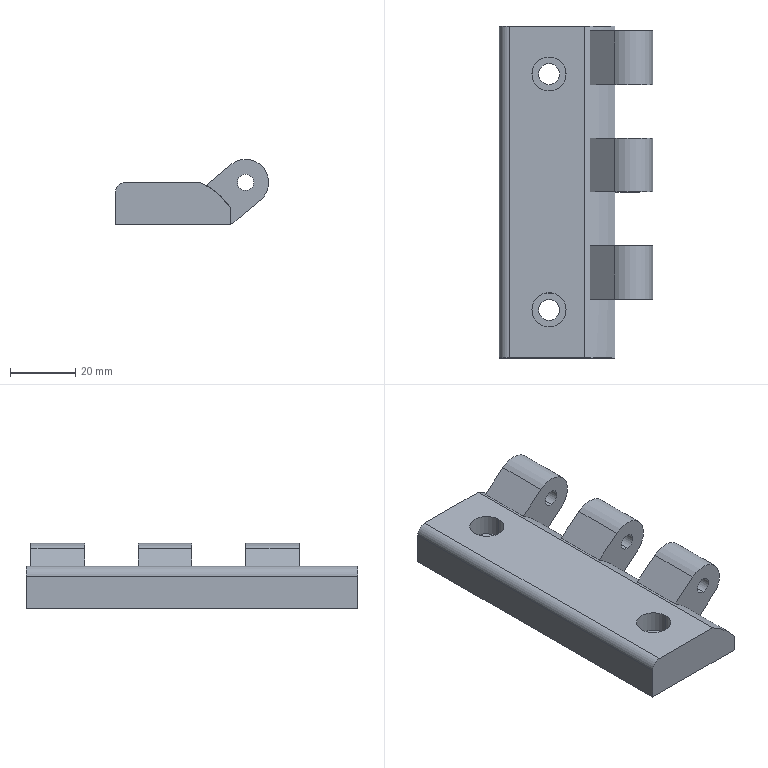Part | SolidWorks | features MBimport 1 | 1 solid | 42 faces | box 47.1 x 102 x 20.1 mm | volume 51608 mm3 | plane 23 | cylinder 19 | commonest cylinder face diameters 5 x6 6.5 x4 10.5 x4 14.2 x3 6 x1 49.62 x1
STEP:
#1=CARTESIAN_POINT('',(-28.,-36.25,-6.5));
#2=VERTEX_POINT('',#1);
#3=CARTESIAN_POINT('',(-21.5,-36.25,-6.5));
#4=VERTEX_POINT('',#3);
#5=CARTESIAN_POINT('',(-24.75,-36.25,-6.5));
#6=DIRECTION('',(0.,0.,-1.));
#7=DIRECTION('',(-1.,0.,0.));
#8=AXIS2_PLACEMENT_3D('',#5,#6,#7);
#9=CIRCLE('',#8,3.25);
#10=EDGE_CURVE('',#2,#4,#9,.T.);
#11=ORIENTED_EDGE('',*,*,#10,.F.);
#12=CARTESIAN_POINT('',(-28.,-36.25,-13.));
#13=VERTEX_POINT('',#12);
#14=CARTESIAN_POINT('',(-28.,-36.25,0.));
#15=DIRECTION('',(0.,0.,-1.));
#16=VECTOR('',#15,1000.);
#17=LINE('',#14,#16);
#18=EDGE_CURVE('',#2,#13,#17,.T.);
#19=ORIENTED_EDGE('',*,*,#18,.T.);
#20=CARTESIAN_POINT('',(-21.5,-36.25,-13.));
#21=VERTEX_POINT('',#20);
#22=CARTESIAN_POINT('',(-24.75,-36.25,-13.));
#23=DIRECTION('',(0.,0.,1.));
#24=DIRECTION('',(1.,0.,0.));
#25=AXIS2_PLACEMENT_3D('',#22,#23,#24);
#26=CIRCLE('',#25,3.25);
#27=EDGE_CURVE('',#21,#13,#26,.T.);
#28=ORIENTED_EDGE('',*,*,#27,.F.);
#29=CARTESIAN_POINT('',(-21.5,-36.25,0.));
#30=DIRECTION('',(0.,0.,-1.));
#31=VECTOR('',#30,1000.);
#32=LINE('',#29,#31);
#33=EDGE_CURVE('',#4,#21,#32,.T.);
#34=ORIENTED_EDGE('',*,*,#33,.F.);
#35=EDGE_LOOP('',(#11,#19,#28,#34));
#36=FACE_OUTER_BOUND('',#35,.T.);
#37=CARTESIAN_POINT('',(-24.75,-36.25,0.));
#38=DIRECTION('',(0.,0.,-1.));
#39=DIRECTION('',(1.,0.,0.));
#40=AXIS2_PLACEMENT_3D('',#37,#38,#39);
#41=CYLINDRICAL_SURFACE('',#40,3.25);
#42=ADVANCED_FACE('',(#36),#41,.F.);
#43=CARTESIAN_POINT('',(-28.,36.25,-6.5));
#44=VERTEX_POINT('',#43);
#45=CARTESIAN_POINT('',(-21.5,36.25,-6.5));
#46=VERTEX_POINT('',#45);
#47=CARTESIAN_POINT('',(-24.75,36.25,-6.5));
#48=DIRECTION('',(0.,0.,-1.));
#49=DIRECTION('',(-1.,0.,0.));
#50=AXIS2_PLACEMENT_3D('',#47,#48,#49);
#51=CIRCLE('',#50,3.25);
#52=EDGE_CURVE('',#44,#46,#51,.T.);
#53=ORIENTED_EDGE('',*,*,#52,.F.);
#54=CARTESIAN_POINT('',(-28.,36.25,-13.));
#55=VERTEX_POINT('',#54);
#56=CARTESIAN_POINT('',(-28.,36.25,0.));
#57=DIRECTION('',(0.,0.,-1.));
#58=VECTOR('',#57,1000.);
#59=LINE('',#56,#58);
#60=EDGE_CURVE('',#44,#55,#59,.T.);
#61=ORIENTED_EDGE('',*,*,#60,.T.);
#62=CARTESIAN_POINT('',(-21.5,36.25,-13.));
#63=VERTEX_POINT('',#62);
#64=CARTESIAN_POINT('',(-24.75,36.25,-13.));
#65=DIRECTION('',(0.,0.,1.));
#66=DIRECTION('',(1.,0.,0.));
#67=AXIS2_PLACEMENT_3D('',#64,#65,#66);
#68=CIRCLE('',#67,3.25);
#69=EDGE_CURVE('',#63,#55,#68,.T.);
#70=ORIENTED_EDGE('',*,*,#69,.F.);
#71=CARTESIAN_POINT('',(-21.5,36.25,0.));
#72=DIRECTION('',(0.,0.,-1.));
#73=VECTOR('',#72,1000.);
#74=LINE('',#71,#73);
#75=EDGE_CURVE('',#46,#63,#74,.T.);
#76=ORIENTED_EDGE('',*,*,#75,.F.);
#77=EDGE_LOOP('',(#53,#61,#70,#76));
#78=FACE_OUTER_BOUND('',#77,.T.);
#79=CARTESIAN_POINT('',(-24.75,36.25,0.));
#80=DIRECTION('',(0.,0.,-1.));
#81=DIRECTION('',(1.,0.,0.));
#82=AXIS2_PLACEMENT_3D('',#79,#80,#81);
#83=CYLINDRICAL_SURFACE('',#82,3.25);
#84=ADVANCED_FACE('',(#78),#83,.F.);
#85=CARTESIAN_POINT('',(-30.,-36.25,0.));
#86=VERTEX_POINT('',#85);
#87=CARTESIAN_POINT('',(-19.5,-36.25,0.));
#88=VERTEX_POINT('',#87);
#89=CARTESIAN_POINT('',(-24.75,-36.25,0.));
#90=DIRECTION('',(0.,0.,-1.));
#91=DIRECTION('',(1.,0.,0.));
#92=AXIS2_PLACEMENT_3D('',#89,#90,#91);
#93=CIRCLE('',#92,5.25);
#94=EDGE_CURVE('',#86,#88,#93,.T.);
#95=ORIENTED_EDGE('',*,*,#94,.F.);
#96=CARTESIAN_POINT('',(-30.,-36.25,-6.5));
#97=VERTEX_POINT('',#96);
#98=CARTESIAN_POINT('',(-30.,-36.25,0.));
#99=DIRECTION('',(0.,0.,-1.));
#100=VECTOR('',#99,1000.);
#101=LINE('',#98,#100);
#102=EDGE_CURVE('',#86,#97,#101,.T.);
#103=ORIENTED_EDGE('',*,*,#102,.T.);
#104=CARTESIAN_POINT('',(-19.5,-36.25,-6.5));
#105=VERTEX_POINT('',#104);
#106=CARTESIAN_POINT('',(-24.75,-36.25,-6.5));
#107=DIRECTION('',(0.,0.,1.));
#108=DIRECTION('',(1.,0.,0.));
#109=AXIS2_PLACEMENT_3D('',#106,#107,#108);
#110=CIRCLE('',#109,5.25);
#111=EDGE_CURVE('',#105,#97,#110,.T.);
#112=ORIENTED_EDGE('',*,*,#111,.F.);
#113=CARTESIAN_POINT('',(-19.5,-36.25,0.));
#114=DIRECTION('',(0.,0.,-1.));
#115=VECTOR('',#114,1000.);
#116=LINE('',#113,#115);
#117=EDGE_CURVE('',#88,#105,#116,.T.);
#118=ORIENTED_EDGE('',*,*,#117,.F.);
#119=EDGE_LOOP('',(#95,#103,#112,#118));
#120=FACE_OUTER_BOUND('',#119,.T.);
#121=CARTESIAN_POINT('',(-24.75,-36.25,0.));
#122=DIRECTION('',(0.,0.,-1.));
#123=DIRECTION('',(1.,0.,0.));
#124=AXIS2_PLACEMENT_3D('',#121,#122,#123);
#125=CYLINDRICAL_SURFACE('',#124,5.25);
#126=ADVANCED_FACE('',(#120),#125,.F.);
#127=CARTESIAN_POINT('',(-30.,36.25,0.));
#128=VERTEX_POINT('',#127);
#129=CARTESIAN_POINT('',(-19.5,36.25,0.));
#130=VERTEX_POINT('',#129);
#131=CARTESIAN_POINT('',(-24.75,36.25,0.));
#132=DIRECTION('',(0.,0.,-1.));
#133=DIRECTION('',(1.,0.,0.));
#134=AXIS2_PLACEMENT_3D('',#131,#132,#133);
#135=CIRCLE('',#134,5.25);
#136=EDGE_CURVE('',#128,#130,#135,.T.);
#137=ORIENTED_EDGE('',*,*,#136,.F.);
#138=CARTESIAN_POINT('',(-30.,36.25,-6.5));
#139=VERTEX_POINT('',#138);
#140=CARTESIAN_POINT('',(-30.,36.25,0.));
#141=DIRECTION('',(0.,0.,-1.));
#142=VECTOR('',#141,1000.);
#143=LINE('',#140,#142);
#144=EDGE_CURVE('',#128,#139,#143,.T.);
#145=ORIENTED_EDGE('',*,*,#144,.T.);
#146=CARTESIAN_POINT('',(-19.5,36.25,-6.5));
#147=VERTEX_POINT('',#146);
#148=CARTESIAN_POINT('',(-24.75,36.25,-6.5));
#149=DIRECTION('',(0.,0.,1.));
#150=DIRECTION('',(1.,0.,0.));
#151=AXIS2_PLACEMENT_3D('',#148,#149,#150);
#152=CIRCLE('',#151,5.25);
#153=EDGE_CURVE('',#147,#139,#152,.T.);
#154=ORIENTED_EDGE('',*,*,#153,.F.);
#155=CARTESIAN_POINT('',(-19.5,36.25,0.));
#156=DIRECTION('',(0.,0.,-1.));
#157=VECTOR('',#156,1000.);
#158=LINE('',#155,#157);
#159=EDGE_CURVE('',#130,#147,#158,.T.);
#160=ORIENTED_EDGE('',*,*,#159,.F.);
#161=EDGE_LOOP('',(#137,#145,#154,#160));
#162=FACE_OUTER_BOUND('',#161,.T.);
#163=CARTESIAN_POINT('',(-24.75,36.25,0.));
#164=DIRECTION('',(0.,0.,-1.));
#165=DIRECTION('',(1.,0.,0.));
#166=AXIS2_PLACEMENT_3D('',#163,#164,#165);
#167=CYLINDRICAL_SURFACE('',#166,5.25);
#168=ADVANCED_FACE('',(#162),#167,.F.);
#169=CARTESIAN_POINT('',(0.,49.5,-2.5));
#170=VERTEX_POINT('',#169);
#171=CARTESIAN_POINT('',(0.,49.5,2.5));
#172=VERTEX_POINT('',#171);
#173=CARTESIAN_POINT('',(0.,49.5,0.));
#174=DIRECTION('',(0.,1.,0.));
#175=DIRECTION('',(1.,0.,0.));
#176=AXIS2_PLACEMENT_3D('',#173,#174,#175);
#177=CIRCLE('',#176,2.5);
#178=EDGE_CURVE('',#170,#172,#177,.T.);
#179=ORIENTED_EDGE('',*,*,#178,.T.);
#180=CARTESIAN_POINT('',(0.,33.,2.5));
#181=VERTEX_POINT('',#180);
#182=CARTESIAN_POINT('',(0.,49.5,2.5));
#183=DIRECTION('',(0.,-1.,0.));
#184=VECTOR('',#183,1000.);
#185=LINE('',#182,#184);
#186=EDGE_CURVE('',#172,#181,#185,.T.);
#187=ORIENTED_EDGE('',*,*,#186,.T.);
#188=CARTESIAN_POINT('',(0.,33.,-2.5));
#189=VERTEX_POINT('',#188);
#190=CARTESIAN_POINT('',(0.,33.,0.));
#191=DIRECTION('',(0.,1.,0.));
#192=DIRECTION('',(1.,0.,0.));
#193=AXIS2_PLACEMENT_3D('',#190,#191,#192);
#194=CIRCLE('',#193,2.5);
#195=EDGE_CURVE('',#189,#181,#194,.T.);
#196=ORIENTED_EDGE('',*,*,#195,.F.);
#197=CARTESIAN_POINT('',(0.,49.5,-2.5));
#198=DIRECTION('',(0.,-1.,0.));
#199=VECTOR('',#198,1000.);
#200=LINE('',#197,#199);
#201=EDGE_CURVE('',#170,#189,#200,.T.);
#202=ORIENTED_EDGE('',*,*,#201,.F.);
#203=EDGE_LOOP('',(#179,#187,#196,#202));
#204=FACE_OUTER_BOUND('',#203,.T.);
#205=CARTESIAN_POINT('',(0.,49.5,0.));
#206=DIRECTION('',(0.,-1.,0.));
#207=DIRECTION('',(0.,0.,-1.));
#208=AXIS2_PLACEMENT_3D('',#205,#206,#207);
#209=CYLINDRICAL_SURFACE('',#208,2.5);
#210=ADVANCED_FACE('',(#204),#209,.F.);
#211=CARTESIAN_POINT('',(0.,16.5,-2.5));
#212=VERTEX_POINT('',#211);
#213=CARTESIAN_POINT('',(0.,16.5,2.5));
#214=VERTEX_POINT('',#213);
#215=CARTESIAN_POINT('',(0.,16.5,0.));
#216=DIRECTION('',(0.,1.,0.));
#217=DIRECTION('',(1.,0.,0.));
#218=AXIS2_PLACEMENT_3D('',#215,#216,#217);
#219=CIRCLE('',#218,2.5);
#220=EDGE_CURVE('',#212,#214,#219,.T.);
#221=ORIENTED_EDGE('',*,*,#220,.T.);
#222=CARTESIAN_POINT('',(0.,0.,2.5));
#223=VERTEX_POINT('',#222);
#224=CARTESIAN_POINT('',(0.,16.5,2.5));
#225=DIRECTION('',(0.,-1.,0.));
#226=VECTOR('',#225,1000.);
#227=LINE('',#224,#226);
#228=EDGE_CURVE('',#214,#223,#227,.T.);
#229=ORIENTED_EDGE('',*,*,#228,.T.);
#230=CARTESIAN_POINT('',(0.,0.,-2.5));
#231=VERTEX_POINT('',#230);
#232=CARTESIAN_POINT('',(0.,0.,0.));
#233=DIRECTION('',(0.,1.,0.));
#234=DIRECTION('',(1.,0.,0.));
#235=AXIS2_PLACEMENT_3D('',#232,#233,#234);
#236=CIRCLE('',#235,2.5);
#237=EDGE_CURVE('',#231,#223,#236,.T.);
#238=ORIENTED_EDGE('',*,*,#237,.F.);
#239=CARTESIAN_POINT('',(0.,16.5,-2.5));
#240=DIRECTION('',(0.,-1.,0.));
#241=VECTOR('',#240,1000.);
#242=LINE('',#239,#241);
#243=EDGE_CURVE('',#212,#231,#242,.T.);
#244=ORIENTED_EDGE('',*,*,#243,.F.);
#245=EDGE_LOOP('',(#221,#229,#238,#244));
#246=FACE_OUTER_BOUND('',#245,.T.);
#247=CARTESIAN_POINT('',(0.,16.5,0.));
#248=DIRECTION('',(0.,-1.,0.));
#249=DIRECTION('',(0.,0.,-1.));
#250=AXIS2_PLACEMENT_3D('',#247,#248,#249);
#251=CYLINDRICAL_SURFACE('',#250,2.5);
#252=ADVANCED_FACE('',(#246),#251,.F.);
#253=CARTESIAN_POINT('',(0.,-16.5,-2.5));
#254=VERTEX_POINT('',#253);
#255=CARTESIAN_POINT('',(0.,-16.5,2.5));
#256=VERTEX_POINT('',#255);
#257=CARTESIAN_POINT('',(0.,-16.5,0.));
#258=DIRECTION('',(0.,1.,0.));
#259=DIRECTION('',(1.,0.,0.));
#260=AXIS2_PLACEMENT_3D('',#257,#258,#259);
#261=CIRCLE('',#260,2.5);
#262=EDGE_CURVE('',#254,#256,#261,.T.);
#263=ORIENTED_EDGE('',*,*,#262,.T.);
#264=CARTESIAN_POINT('',(0.,-33.,2.5));
#265=VERTEX_POINT('',#264);
#266=CARTESIAN_POINT('',(0.,-16.5,2.5));
#267=DIRECTION('',(0.,-1.,0.));
#268=VECTOR('',#267,1000.);
#269=LINE('',#266,#268);
#270=EDGE_CURVE('',#256,#265,#269,.T.);
#271=ORIENTED_EDGE('',*,*,#270,.T.);
#272=CARTESIAN_POINT('',(0.,-33.,-2.5));
#273=VERTEX_POINT('',#272);
#274=CARTESIAN_POINT('',(0.,-33.,0.));
#275=DIRECTION('',(0.,1.,0.));
#276=DIRECTION('',(1.,0.,0.));
#277=AXIS2_PLACEMENT_3D('',#274,#275,#276);
#278=CIRCLE('',#277,2.5);
#279=EDGE_CURVE('',#273,#265,#278,.T.);
#280=ORIENTED_EDGE('',*,*,#279,.F.);
#281=CARTESIAN_POINT('',(0.,-16.5,-2.5));
#282=DIRECTION('',(0.,-1.,0.));
#283=VECTOR('',#282,1000.);
#284=LINE('',#281,#283);
#285=EDGE_CURVE('',#254,#273,#284,.T.);
#286=ORIENTED_EDGE('',*,*,#285,.F.);
#287=EDGE_LOOP('',(#263,#271,#280,#286));
#288=FACE_OUTER_BOUND('',#287,.T.);
#289=CARTESIAN_POINT('',(0.,-16.5,0.));
#290=DIRECTION('',(0.,-1.,0.));
#291=DIRECTION('',(0.,0.,-1.));
#292=AXIS2_PLACEMENT_3D('',#289,#290,#291);
#293=CYLINDRICAL_SURFACE('',#292,2.5);
#294=ADVANCED_FACE('',(#288),#293,.F.);
#295=CARTESIAN_POINT('',(-4.5,49.5,-7.958));
#296=VERTEX_POINT('',#295);
#297=CARTESIAN_POINT('',(-12.154,49.5,-0.8929));
#298=VERTEX_POINT('',#297);
#299=CARTESIAN_POINT('',(-24.78,49.5,-22.25));
#300=DIRECTION('',(0.,-1.,0.));
#301=DIRECTION('',(1.,0.,0.));
#302=AXIS2_PLACEMENT_3D('',#299,#300,#301);
#303=CIRCLE('',#302,24.81);
#304=EDGE_CURVE('',#296,#298,#303,.T.);
#305=ORIENTED_EDGE('',*,*,#304,.F.);
#306=CARTESIAN_POINT('',(-4.5,51.,-7.958));
#307=VERTEX_POINT('',#306);
#308=CARTESIAN_POINT('',(-4.5,-51.,-7.958));
#309=DIRECTION('',(0.,1.,0.));
#310=VECTOR('',#309,1000.);
#311=LINE('',#308,#310);
#312=EDGE_CURVE('',#296,#307,#311,.T.);
#313=ORIENTED_EDGE('',*,*,#312,.T.);
#314=CARTESIAN_POINT('',(-13.804,51.,0.));
#315=VERTEX_POINT('',#314);
#316=CARTESIAN_POINT('',(-24.78,51.,-22.25));
#317=DIRECTION('',(0.,-1.,0.));
#318=DIRECTION('',(1.,0.,0.));
#319=AXIS2_PLACEMENT_3D('',#316,#317,#318);
#320=CIRCLE('',#319,24.81);
#321=EDGE_CURVE('',#307,#315,#320,.T.);
#322=ORIENTED_EDGE('',*,*,#321,.T.);
#323=CARTESIAN_POINT('',(-13.804,-51.,0.));
#324=VERTEX_POINT('',#323);
#325=CARTESIAN_POINT('',(-13.804,-51.,0.));
#326=DIRECTION('',(0.,1.,0.));
#327=VECTOR('',#326,1000.);
#328=LINE('',#325,#327);
#329=EDGE_CURVE('',#324,#315,#328,.T.);
#330=ORIENTED_EDGE('',*,*,#329,.F.);
#331=CARTESIAN_POINT('',(-4.5,-51.,-7.958));
#332=VERTEX_POINT('',#331);
#333=CARTESIAN_POINT('',(-24.78,-51.,-22.25));
#334=DIRECTION('',(0.,-1.,0.));
#335=DIRECTION('',(1.,0.,0.));
#336=AXIS2_PLACEMENT_3D('',#333,#334,#335);
#337=CIRCLE('',#336,24.81);
#338=EDGE_CURVE('',#332,#324,#337,.T.);
#339=ORIENTED_EDGE('',*,*,#338,.F.);
#340=CARTESIAN_POINT('',(-4.5,-33.,-7.958));
#341=VERTEX_POINT('',#340);
#342=CARTESIAN_POINT('',(-4.5,-51.,-7.958));
#343=DIRECTION('',(0.,1.,0.));
#344=VECTOR('',#343,1000.);
#345=LINE('',#342,#344);
#346=EDGE_CURVE('',#332,#341,#345,.T.);
#347=ORIENTED_EDGE('',*,*,#346,.T.);
#348=CARTESIAN_POINT('',(-12.154,-33.,-0.8929));
#349=VERTEX_POINT('',#348);
#350=CARTESIAN_POINT('',(-24.78,-33.,-22.25));
#351=DIRECTION('',(0.,-1.,0.));
#352=DIRECTION('',(1.,0.,0.));
#353=AXIS2_PLACEMENT_3D('',#350,#351,#352);
#354=CIRCLE('',#353,24.81);
#355=EDGE_CURVE('',#341,#349,#354,.T.);
#356=ORIENTED_EDGE('',*,*,#355,.T.);
#357=CARTESIAN_POINT('',(-12.154,-16.5,-0.8929));
#358=VERTEX_POINT('',#357);
#359=CARTESIAN_POINT('',(-12.154,-16.5,-0.8929));
#360=DIRECTION('',(0.,-1.,0.));
#361=VECTOR('',#360,1000.);
#362=LINE('',#359,#361);
#363=EDGE_CURVE('',#358,#349,#362,.T.);
#364=ORIENTED_EDGE('',*,*,#363,.F.);
#365=CARTESIAN_POINT('',(-4.5,-16.5,-7.958));
#366=VERTEX_POINT('',#365);
#367=CARTESIAN_POINT('',(-24.78,-16.5,-22.25));
#368=DIRECTION('',(0.,-1.,0.));
#369=DIRECTION('',(1.,0.,0.));
#370=AXIS2_PLACEMENT_3D('',#367,#368,#369);
#371=CIRCLE('',#370,24.81);
#372=EDGE_CURVE('',#366,#358,#371,.T.);
#373=ORIENTED_EDGE('',*,*,#372,.F.);
#374=CARTESIAN_POINT('',(-4.5,0.,-7.958));
#375=VERTEX_POINT('',#374);
#376=CARTESIAN_POINT('',(-4.5,-51.,-7.958));
#377=DIRECTION('',(0.,1.,0.));
#378=VECTOR('',#377,1000.);
#379=LINE('',#376,#378);
#380=EDGE_CURVE('',#366,#375,#379,.T.);
#381=ORIENTED_EDGE('',*,*,#380,.T.);
#382=CARTESIAN_POINT('',(-12.154,0.,-0.8929));
#383=VERTEX_POINT('',#382);
#384=CARTESIAN_POINT('',(-24.78,0.,-22.25));
#385=DIRECTION('',(0.,-1.,0.));
#386=DIRECTION('',(1.,0.,0.));
#387=AXIS2_PLACEMENT_3D('',#384,#385,#386);
#388=CIRCLE('',#387,24.81);
#389=EDGE_CURVE('',#375,#383,#388,.T.);
#390=ORIENTED_EDGE('',*,*,#389,.T.);
#391=CARTESIAN_POINT('',(-12.154,16.5,-0.8929));
#392=VERTEX_POINT('',#391);
#393=CARTESIAN_POINT('',(-12.154,16.5,-0.8929));
#394=DIRECTION('',(0.,-1.,0.));
#395=VECTOR('',#394,1000.);
#396=LINE('',#393,#395);
#397=EDGE_CURVE('',#392,#383,#396,.T.);
#398=ORIENTED_EDGE('',*,*,#397,.F.);
#399=CARTESIAN_POINT('',(-4.5,16.5,-7.958));
#400=VERTEX_POINT('',#399);
#401=CARTESIAN_POINT('',(-24.78,16.5,-22.25));
#402=DIRECTION('',(0.,-1.,0.));
#403=DIRECTION('',(1.,0.,0.));
#404=AXIS2_PLACEMENT_3D('',#401,#402,#403);
#405=CIRCLE('',#404,24.81);
#406=EDGE_CURVE('',#400,#392,#405,.T.);
#407=ORIENTED_EDGE('',*,*,#406,.F.);
#408=CARTESIAN_POINT('',(-4.5,33.,-7.958));
#409=VERTEX_POINT('',#408);
#410=CARTESIAN_POINT('',(-4.5,-51.,-7.958));
#411=DIRECTION('',(0.,1.,0.));
#412=VECTOR('',#411,1000.);
#413=LINE('',#410,#412);
#414=EDGE_CURVE('',#400,#409,#413,.T.);
#415=ORIENTED_EDGE('',*,*,#414,.T.);
#416=CARTESIAN_POINT('',(-12.154,33.,-0.8929));
#417=VERTEX_POINT('',#416);
#418=CARTESIAN_POINT('',(-24.78,33.,-22.25));
#419=DIRECTION('',(0.,-1.,0.));
#420=DIRECTION('',(1.,0.,0.));
#421=AXIS2_PLACEMENT_3D('',#418,#419,#420);
#422=CIRCLE('',#421,24.81);
#423=EDGE_CURVE('',#409,#417,#422,.T.);
#424=ORIENTED_EDGE('',*,*,#423,.T.);
#425=CARTESIAN_POINT('',(-12.154,49.5,-0.8929));
#426=DIRECTION('',(0.,-1.,0.));
#427=VECTOR('',#426,1000.);
#428=LINE('',#425,#427);
#429=EDGE_CURVE('',#298,#417,#428,.T.);
#430=ORIENTED_EDGE('',*,*,#429,.F.);
#431=EDGE_LOOP('',(#305,#313,#322,#330,#339,#347,#356,#364,#373,#381,#390,#398,#407,#415,#424,#430));
#432=FACE_OUTER_BOUND('',#431,.T.);
#433=CARTESIAN_POINT('',(-24.78,-51.,-22.25));
#434=DIRECTION('',(0.,1.,0.));
#435=DIRECTION('',(0.,0.,1.));
#436=AXIS2_PLACEMENT_3D('',#433,#434,#435);
#437=CYLINDRICAL_SURFACE('',#436,24.81);
#438=ADVANCED_FACE('',(#432),#437,.T.);
#439=CARTESIAN_POINT('',(-4.5,49.5,-13.));
#440=VERTEX_POINT('',#439);
#441=CARTESIAN_POINT('',(-4.5,49.5,-13.));
#442=DIRECTION('',(0.,0.,1.));
#443=VECTOR('',#442,1000.);
#444=LINE('',#441,#443);
#445=EDGE_CURVE('',#440,#296,#444,.T.);
#446=ORIENTED_EDGE('',*,*,#445,.F.);
#447=CARTESIAN_POINT('',(-4.5,51.,-13.));
#448=VERTEX_POINT('',#447);
#449=CARTESIAN_POINT('',(-4.5,-51.,-13.));
#450=DIRECTION('',(0.,1.,0.));
#451=VECTOR('',#450,1000.);
#452=LINE('',#449,#451);
#453=EDGE_CURVE('',#440,#448,#452,.T.);
#454=ORIENTED_EDGE('',*,*,#453,.T.);
#455=CARTESIAN_POINT('',(-4.5,51.,-13.));
#456=DIRECTION('',(0.,0.,1.));
#457=VECTOR('',#456,1000.);
#458=LINE('',#455,#457);
#459=EDGE_CURVE('',#448,#307,#458,.T.);
#460=ORIENTED_EDGE('',*,*,#459,.T.);
#461=ORIENTED_EDGE('',*,*,#312,.F.);
#462=EDGE_LOOP('',(#446,#454,#460,#461));
#463=FACE_OUTER_BOUND('',#462,.T.);
#464=CARTESIAN_POINT('',(-4.5,-51.,-13.));
#465=DIRECTION('',(-1.,0.,0.));
#466=DIRECTION('',(0.,0.,1.));
#467=AXIS2_PLACEMENT_3D('',#464,#465,#466);
#468=PLANE('',#467);
#469=ADVANCED_FACE('',(#463),#468,.F.);
#470=CARTESIAN_POINT('',(-4.5,16.5,-13.));
#471=VERTEX_POINT('',#470);
#472=CARTESIAN_POINT('',(-4.5,33.,-13.));
#473=VERTEX_POINT('',#472);
#474=CARTESIAN_POINT('',(-4.5,-51.,-13.));
#475=DIRECTION('',(0.,1.,0.));
#476=VECTOR('',#475,1000.);
#477=LINE('',#474,#476);
#478=EDGE_CURVE('',#471,#473,#477,.T.);
#479=ORIENTED_EDGE('',*,*,#478,.T.);
#480=CARTESIAN_POINT('',(-4.5,33.,-13.));
#481=DIRECTION('',(0.,0.,1.));
#482=VECTOR('',#481,1000.);
#483=LINE('',#480,#482);
#484=EDGE_CURVE('',#473,#409,#483,.T.);
#485=ORIENTED_EDGE('',*,*,#484,.T.);
#486=ORIENTED_EDGE('',*,*,#414,.F.);
#487=CARTESIAN_POINT('',(-4.5,16.5,-13.));
#488=DIRECTION('',(0.,0.,1.));
#489=VECTOR('',#488,1000.);
#490=LINE('',#487,#489);
#491=EDGE_CURVE('',#471,#400,#490,.T.);
#492=ORIENTED_EDGE('',*,*,#491,.F.);
#493=EDGE_LOOP('',(#479,#485,#486,#492));
#494=FACE_OUTER_BOUND('',#493,.T.);
#495=CARTESIAN_POINT('',(-4.5,-51.,-13.));
#496=DIRECTION('',(-1.,0.,0.));
#497=DIRECTION('',(0.,0.,1.));
#498=AXIS2_PLACEMENT_3D('',#495,#496,#497);
#499=PLANE('',#498);
#500=ADVANCED_FACE('',(#494),#499,.F.);
#501=CARTESIAN_POINT('',(-4.5,-16.5,-13.));
#502=VERTEX_POINT('',#501);
#503=CARTESIAN_POINT('',(-4.5,0.,-13.));
#504=VERTEX_POINT('',#503);
#505=CARTESIAN_POINT('',(-4.5,-51.,-13.));
#506=DIRECTION('',(0.,1.,0.));
#507=VECTOR('',#506,1000.);
#508=LINE('',#505,#507);
#509=EDGE_CURVE('',#502,#504,#508,.T.);
#510=ORIENTED_EDGE('',*,*,#509,.T.);
#511=CARTESIAN_POINT('',(-4.5,0.,-13.));
#512=DIRECTION('',(0.,0.,1.));
#513=VECTOR('',#512,1000.);
#514=LINE('',#511,#513);
#515=EDGE_CURVE('',#504,#375,#514,.T.);
#516=ORIENTED_EDGE('',*,*,#515,.T.);
#517=ORIENTED_EDGE('',*,*,#380,.F.);
#518=CARTESIAN_POINT('',(-4.5,-16.5,-13.));
#519=DIRECTION('',(0.,0.,1.));
#520=VECTOR('',#519,1000.);
#521=LINE('',#518,#520);
#522=EDGE_CURVE('',#502,#366,#521,.T.);
#523=ORIENTED_EDGE('',*,*,#522,.F.);
#524=EDGE_LOOP('',(#510,#516,#517,#523));
#525=FACE_OUTER_BOUND('',#524,.T.);
#526=CARTESIAN_POINT('',(-4.5,-51.,-13.));
#527=DIRECTION('',(-1.,0.,0.));
#528=DIRECTION('',(0.,0.,1.));
#529=AXIS2_PLACEMENT_3D('',#526,#527,#528);
#530=PLANE('',#529);
#531=ADVANCED_FACE('',(#525),#530,.F.);
#532=CARTESIAN_POINT('',(-24.75,-36.25,0.));
#533=DIRECTION('',(0.,0.,-1.));
#534=DIRECTION('',(1.,0.,0.));
#535=AXIS2_PLACEMENT_3D('',#532,#533,#534);
#536=CIRCLE('',#535,5.25);
#537=EDGE_CURVE('',#88,#86,#536,.T.);
#538=ORIENTED_EDGE('',*,*,#537,.T.);
#539=ORIENTED_EDGE('',*,*,#94,.T.);
#540=EDGE_LOOP('',(#538,#539));
#541=FACE_BOUND('',#540,.T.);
#542=CARTESIAN_POINT('',(-24.75,36.25,0.));
#543=DIRECTION('',(0.,0.,-1.));
#544=DIRECTION('',(1.,0.,0.));
#545=AXIS2_PLACEMENT_3D('',#542,#543,#544);
#546=CIRCLE('',#545,5.25);
#547=EDGE_CURVE('',#130,#128,#546,.T.);
#548=ORIENTED_EDGE('',*,*,#547,.T.);
#549=ORIENTED_EDGE('',*,*,#136,.T.);
#550=EDGE_LOOP('',(#548,#549));
#551=FACE_BOUND('',#550,.T.);
#552=CARTESIAN_POINT('',(-37.,51.,0.));
#553=VERTEX_POINT('',#552);
#554=CARTESIAN_POINT('',(-13.804,51.,0.));
#555=DIRECTION('',(-1.,0.,0.));
#556=VECTOR('',#555,1000.);
#557=LINE('',#554,#556);
#558=EDGE_CURVE('',#315,#553,#557,.T.);
#559=ORIENTED_EDGE('',*,*,#558,.T.);
#560=CARTESIAN_POINT('',(-37.,-51.,0.));
#561=VERTEX_POINT('',#560);
#562=CARTESIAN_POINT('',(-37.,-51.,0.));
#563=DIRECTION('',(0.,-1.,0.));
#564=VECTOR('',#563,1000.);
#565=LINE('',#562,#564);
#566=EDGE_CURVE('',#553,#561,#565,.T.);
#567=ORIENTED_EDGE('',*,*,#566,.T.);
#568=CARTESIAN_POINT('',(-13.804,-51.,0.));
#569=DIRECTION('',(-1.,0.,0.));
#570=VECTOR('',#569,1000.);
#571=LINE('',#568,#570);
#572=EDGE_CURVE('',#324,#561,#571,.T.);
#573=ORIENTED_EDGE('',*,*,#572,.F.);
#574=ORIENTED_EDGE('',*,*,#329,.T.);
#575=EDGE_LOOP('',(#559,#567,#573,#574));
#576=FACE_OUTER_BOUND('',#575,.T.);
#577=CARTESIAN_POINT('',(-13.804,-51.,0.));
#578=DIRECTION('',(0.,0.,-1.));
#579=DIRECTION('',(0.,-1.,0.));
#580=AXIS2_PLACEMENT_3D('',#577,#578,#579);
#581=PLANE('',#580);
#582=ADVANCED_FACE('',(#541,#551,#576),#581,.F.);
#583=CARTESIAN_POINT('',(-40.,-51.,-3.));
#584=VERTEX_POINT('',#583);
#585=CARTESIAN_POINT('',(-40.,-51.,-13.));
#586=VERTEX_POINT('',#585);
#587=CARTESIAN_POINT('',(-40.,-51.,0.));
#588=DIRECTION('',(0.,0.,-1.));
#589=VECTOR('',#588,1000.);
#590=LINE('',#587,#589);
#591=EDGE_CURVE('',#584,#586,#590,.T.);
#592=ORIENTED_EDGE('',*,*,#591,.F.);
#593=CARTESIAN_POINT('',(-40.,51.,-3.));
#594=VERTEX_POINT('',#593);
#595=CARTESIAN_POINT('',(-40.,-51.,-3.));
#596=DIRECTION('',(0.,1.,0.));
#597=VECTOR('',#596,1000.);
#598=LINE('',#595,#597);
#599=EDGE_CURVE('',#584,#594,#598,.T.);
#600=ORIENTED_EDGE('',*,*,#599,.T.);
#601=CARTESIAN_POINT('',(-40.,51.,-13.));
#602=VERTEX_POINT('',#601);
#603=CARTESIAN_POINT('',(-40.,51.,0.));
#604=DIRECTION('',(0.,0.,-1.));
#605=VECTOR('',#604,1000.);
#606=LINE('',#603,#605);
#607=EDGE_CURVE('',#594,#602,#606,.T.);
#608=ORIENTED_EDGE('',*,*,#607,.T.);
#609=CARTESIAN_POINT('',(-40.,-51.,-13.));
#610=DIRECTION('',(0.,1.,0.));
#611=VECTOR('',#610,1000.);
#612=LINE('',#609,#611);
#613=EDGE_CURVE('',#586,#602,#612,.T.);
#614=ORIENTED_EDGE('',*,*,#613,.F.);
#615=EDGE_LOOP('',(#592,#600,#608,#614));
#616=FACE_OUTER_BOUND('',#615,.T.);
#617=CARTESIAN_POINT('',(-40.,-51.,0.));
#618=DIRECTION('',(1.,0.,0.));
#619=DIRECTION('',(0.,1.,0.));
#620=AXIS2_PLACEMENT_3D('',#617,#618,#619);
#621=PLANE('',#620);
#622=ADVANCED_FACE('',(#616),#621,.F.);
#623=ORIENTED_EDGE('',*,*,#27,.T.);
#624=CARTESIAN_POINT('',(-24.75,-36.25,-13.));
#625=DIRECTION('',(0.,0.,1.));
#626=DIRECTION('',(1.,0.,0.));
#627=AXIS2_PLACEMENT_3D('',#624,#625,#626);
#628=CIRCLE('',#627,3.25);
#629=EDGE_CURVE('',#13,#21,#628,.T.);
#630=ORIENTED_EDGE('',*,*,#629,.T.);
#631=EDGE_LOOP('',(#623,#630));
#632=FACE_BOUND('',#631,.T.);
#633=ORIENTED_EDGE('',*,*,#69,.T.);
#634=CARTESIAN_POINT('',(-24.75,36.25,-13.));
#635=DIRECTION('',(0.,0.,1.));
#636=DIRECTION('',(1.,0.,0.));
#637=AXIS2_PLACEMENT_3D('',#634,#635,#636);
#638=CIRCLE('',#637,3.25);
#639=EDGE_CURVE('',#55,#63,#638,.T.);
#640=ORIENTED_EDGE('',*,*,#639,.T.);
#641=EDGE_LOOP('',(#633,#640));
#642=FACE_BOUND('',#641,.T.);
#643=CARTESIAN_POINT('',(-40.,51.,-13.));
#644=DIRECTION('',(1.,0.,0.));
#645=VECTOR('',#644,1000.);
#646=LINE('',#643,#645);
#647=EDGE_CURVE('',#602,#448,#646,.T.);
#648=ORIENTED_EDGE('',*,*,#647,.T.);
#649=ORIENTED_EDGE('',*,*,#453,.F.);
#650=CARTESIAN_POINT('',(-4.5,49.5,-13.));
#651=DIRECTION('',(0.,-1.,0.));
#652=VECTOR('',#651,1000.);
#653=LINE('',#650,#652);
#654=EDGE_CURVE('',#440,#473,#653,.T.);
#655=ORIENTED_EDGE('',*,*,#654,.T.);
#656=ORIENTED_EDGE('',*,*,#478,.F.);
#657=CARTESIAN_POINT('',(-4.5,16.5,-13.));
#658=DIRECTION('',(0.,-1.,0.));
#659=VECTOR('',#658,1000.);
#660=LINE('',#657,#659);
#661=EDGE_CURVE('',#471,#504,#660,.T.);
#662=ORIENTED_EDGE('',*,*,#661,.T.);
#663=ORIENTED_EDGE('',*,*,#509,.F.);
#664=CARTESIAN_POINT('',(-4.5,-33.,-13.));
#665=VERTEX_POINT('',#664);
#666=CARTESIAN_POINT('',(-4.5,-16.5,-13.));
#667=DIRECTION('',(0.,-1.,0.));
#668=VECTOR('',#667,1000.);
#669=LINE('',#666,#668);
#670=EDGE_CURVE('',#502,#665,#669,.T.);
#671=ORIENTED_EDGE('',*,*,#670,.T.);
#672=CARTESIAN_POINT('',(-4.5,-51.,-13.));
#673=VERTEX_POINT('',#672);
#674=CARTESIAN_POINT('',(-4.5,-51.,-13.));
#675=DIRECTION('',(0.,1.,0.));
#676=VECTOR('',#675,1000.);
#677=LINE('',#674,#676);
#678=EDGE_CURVE('',#673,#665,#677,.T.);
#679=ORIENTED_EDGE('',*,*,#678,.F.);
#680=CARTESIAN_POINT('',(-40.,-51.,-13.));
#681=DIRECTION('',(1.,0.,0.));
#682=VECTOR('',#681,1000.);
#683=LINE('',#680,#682);
#684=EDGE_CURVE('',#586,#673,#683,.T.);
#685=ORIENTED_EDGE('',*,*,#684,.F.);
#686=ORIENTED_EDGE('',*,*,#613,.T.);
#687=EDGE_LOOP('',(#648,#649,#655,#656,#662,#663,#671,#679,#685,#686));
#688=FACE_OUTER_BOUND('',#687,.T.);
#689=CARTESIAN_POINT('',(-40.,-51.,-13.));
#690=DIRECTION('',(0.,0.,1.));
#691=DIRECTION('',(1.,0.,0.));
#692=AXIS2_PLACEMENT_3D('',#689,#690,#691);
#693=PLANE('',#692);
#694=ADVANCED_FACE('',(#632,#642,#688),#693,.F.);
#695=ORIENTED_EDGE('',*,*,#678,.T.);
#696=CARTESIAN_POINT('',(-4.5,-33.,-13.));
#697=DIRECTION('',(0.,0.,1.));
#698=VECTOR('',#697,1000.);
#699=LINE('',#696,#698);
#700=EDGE_CURVE('',#665,#341,#699,.T.);
#701=ORIENTED_EDGE('',*,*,#700,.T.);
#702=ORIENTED_EDGE('',*,*,#346,.F.);
#703=CARTESIAN_POINT('',(-4.5,-51.,-13.));
#704=DIRECTION('',(0.,0.,1.));
#705=VECTOR('',#704,1000.);
#706=LINE('',#703,#705);
#707=EDGE_CURVE('',#673,#332,#706,.T.);
#708=ORIENTED_EDGE('',*,*,#707,.F.);
#709=EDGE_LOOP('',(#695,#701,#702,#708));
#710=FACE_OUTER_BOUND('',#709,.T.);
#711=CARTESIAN_POINT('',(-4.5,-51.,-13.));
#712=DIRECTION('',(-1.,0.,0.));
#713=DIRECTION('',(0.,0.,1.));
#714=AXIS2_PLACEMENT_3D('',#711,#712,#713);
#715=PLANE('',#714);
#716=ADVANCED_FACE('',(#710),#715,.F.);
#717=ORIENTED_EDGE('',*,*,#572,.T.);
#718=CARTESIAN_POINT('',(-37.,-51.,-3.));
#719=DIRECTION('',(0.,-1.,0.));
#720=DIRECTION('',(0.,0.,-1.));
#721=AXIS2_PLACEMENT_3D('',#718,#719,#720);
#722=CIRCLE('',#721,3.);
#723=EDGE_CURVE('',#561,#584,#722,.T.);
#724=ORIENTED_EDGE('',*,*,#723,.T.);
#725=ORIENTED_EDGE('',*,*,#591,.T.);
#726=ORIENTED_EDGE('',*,*,#684,.T.);
#727=ORIENTED_EDGE('',*,*,#707,.T.);
#728=ORIENTED_EDGE('',*,*,#338,.T.);
#729=EDGE_LOOP('',(#717,#724,#725,#726,#727,#728));
#730=FACE_OUTER_BOUND('',#729,.T.);
#731=CARTESIAN_POINT('',(-24.78,-51.,-22.25));
#732=DIRECTION('',(0.,-1.,0.));
#733=DIRECTION('',(0.,0.,-1.));
#734=AXIS2_PLACEMENT_3D('',#731,#732,#733);
#735=PLANE('',#734);
#736=ADVANCED_FACE('',(#730),#735,.T.);
#737=ORIENTED_EDGE('',*,*,#607,.F.);
#738=CARTESIAN_POINT('',(-37.,51.,-3.));
#739=DIRECTION('',(0.,1.,0.));
#740=DIRECTION('',(0.,0.,-1.));
#741=AXIS2_PLACEMENT_3D('',#738,#739,#740);
#742=CIRCLE('',#741,3.);
#743=EDGE_CURVE('',#594,#553,#742,.T.);
#744=ORIENTED_EDGE('',*,*,#743,.T.);
#745=ORIENTED_EDGE('',*,*,#558,.F.);
#746=ORIENTED_EDGE('',*,*,#321,.F.);
#747=ORIENTED_EDGE('',*,*,#459,.F.);
#748=ORIENTED_EDGE('',*,*,#647,.F.);
#749=EDGE_LOOP('',(#737,#744,#745,#746,#747,#748));
#750=FACE_OUTER_BOUND('',#749,.T.);
#751=CARTESIAN_POINT('',(-24.78,51.,-22.25));
#752=DIRECTION('',(0.,-1.,0.));
#753=DIRECTION('',(0.,0.,-1.));
#754=AXIS2_PLACEMENT_3D('',#751,#752,#753);
#755=PLANE('',#754);
#756=ADVANCED_FACE('',(#750),#755,.F.);
#757=CARTESIAN_POINT('',(-4.548,-33.,5.452));
#758=VERTEX_POINT('',#757);
#759=CARTESIAN_POINT('',(-4.548,-33.,5.452));
#760=DIRECTION('',(0.7679,0.,0.6406));
#761=VECTOR('',#760,1000.);
#762=LINE('',#759,#761);
#763=EDGE_CURVE('',#349,#758,#762,.T.);
#764=ORIENTED_EDGE('',*,*,#763,.T.);
#765=CARTESIAN_POINT('',(-4.548,-16.5,5.452));
#766=VERTEX_POINT('',#765);
#767=CARTESIAN_POINT('',(-4.548,-16.5,5.452));
#768=DIRECTION('',(0.,-1.,0.));
#769=VECTOR('',#768,1000.);
#770=LINE('',#767,#769);
#771=EDGE_CURVE('',#766,#758,#770,.T.);
#772=ORIENTED_EDGE('',*,*,#771,.F.);
#773=CARTESIAN_POINT('',(-4.548,-16.5,5.452));
#774=DIRECTION('',(0.7679,0.,0.6406));
#775=VECTOR('',#774,1000.);
#776=LINE('',#773,#775);
#777=EDGE_CURVE('',#358,#766,#776,.T.);
#778=ORIENTED_EDGE('',*,*,#777,.F.);
#779=ORIENTED_EDGE('',*,*,#363,.T.);
#780=EDGE_LOOP('',(#764,#772,#778,#779));
#781=FACE_OUTER_BOUND('',#780,.T.);
#782=CARTESIAN_POINT('',(-4.548,-16.5,5.452));
#783=DIRECTION('',(0.6406,0.,-0.7679));
#784=DIRECTION('',(0.,-1.,0.));
#785=AXIS2_PLACEMENT_3D('',#782,#783,#784);
#786=PLANE('',#785);
#787=ADVANCED_FACE('',(#781),#786,.F.);
#788=CARTESIAN_POINT('',(4.548,-33.,-5.452));
#789=VERTEX_POINT('',#788);
#790=CARTESIAN_POINT('',(0.,-33.,0.));
#791=DIRECTION('',(0.,1.,0.));
#792=DIRECTION('',(-1.,0.,0.));
#793=AXIS2_PLACEMENT_3D('',#790,#791,#792);
#794=CIRCLE('',#793,7.1);
#795=EDGE_CURVE('',#758,#789,#794,.T.);
#796=ORIENTED_EDGE('',*,*,#795,.T.);
#797=CARTESIAN_POINT('',(4.548,-16.5,-5.452));
#798=VERTEX_POINT('',#797);
#799=CARTESIAN_POINT('',(4.548,-16.5,-5.452));
#800=DIRECTION('',(0.,-1.,0.));
#801=VECTOR('',#800,1000.);
#802=LINE('',#799,#801);
#803=EDGE_CURVE('',#798,#789,#802,.T.);
#804=ORIENTED_EDGE('',*,*,#803,.F.);
#805=CARTESIAN_POINT('',(0.,-16.5,0.));
#806=DIRECTION('',(0.,1.,0.));
#807=DIRECTION('',(-1.,0.,0.));
#808=AXIS2_PLACEMENT_3D('',#805,#806,#807);
#809=CIRCLE('',#808,7.1);
#810=EDGE_CURVE('',#766,#798,#809,.T.);
#811=ORIENTED_EDGE('',*,*,#810,.F.);
#812=ORIENTED_EDGE('',*,*,#771,.T.);
#813=EDGE_LOOP('',(#796,#804,#811,#812));
#814=FACE_OUTER_BOUND('',#813,.T.);
#815=CARTESIAN_POINT('',(0.,-16.5,0.));
#816=DIRECTION('',(0.,-1.,0.));
#817=DIRECTION('',(0.,0.,-1.));
#818=AXIS2_PLACEMENT_3D('',#815,#816,#817);
#819=CYLINDRICAL_SURFACE('',#818,7.1);
#820=ADVANCED_FACE('',(#814),#819,.T.);
#821=ORIENTED_EDGE('',*,*,#270,.F.);
#822=CARTESIAN_POINT('',(0.,-16.5,0.));
#823=DIRECTION('',(0.,1.,0.));
#824=DIRECTION('',(1.,0.,0.));
#825=AXIS2_PLACEMENT_3D('',#822,#823,#824);
#826=CIRCLE('',#825,2.5);
#827=EDGE_CURVE('',#256,#254,#826,.T.);
#828=ORIENTED_EDGE('',*,*,#827,.T.);
#829=ORIENTED_EDGE('',*,*,#285,.T.);
#830=CARTESIAN_POINT('',(0.,-33.,0.));
#831=DIRECTION('',(0.,1.,0.));
#832=DIRECTION('',(1.,0.,0.));
#833=AXIS2_PLACEMENT_3D('',#830,#831,#832);
#834=CIRCLE('',#833,2.5);
#835=EDGE_CURVE('',#265,#273,#834,.T.);
#836=ORIENTED_EDGE('',*,*,#835,.F.);
#837=EDGE_LOOP('',(#821,#828,#829,#836));
#838=FACE_OUTER_BOUND('',#837,.T.);
#839=CARTESIAN_POINT('',(0.,-16.5,0.));
#840=DIRECTION('',(0.,-1.,0.));
#841=DIRECTION('',(0.,0.,-1.));
#842=AXIS2_PLACEMENT_3D('',#839,#840,#841);
#843=CYLINDRICAL_SURFACE('',#842,2.5);
#844=ADVANCED_FACE('',(#838),#843,.F.);
#845=CARTESIAN_POINT('',(-4.5,-33.,-13.));
#846=DIRECTION('',(-0.7679,0.,-0.6406));
#847=VECTOR('',#846,1000.);
#848=LINE('',#845,#847);
#849=EDGE_CURVE('',#789,#665,#848,.T.);
#850=ORIENTED_EDGE('',*,*,#849,.T.);
#851=ORIENTED_EDGE('',*,*,#670,.F.);
#852=CARTESIAN_POINT('',(-4.5,-16.5,-13.));
#853=DIRECTION('',(-0.7679,0.,-0.6406));
#854=VECTOR('',#853,1000.);
#855=LINE('',#852,#854);
#856=EDGE_CURVE('',#798,#502,#855,.T.);
#857=ORIENTED_EDGE('',*,*,#856,.F.);
#858=ORIENTED_EDGE('',*,*,#803,.T.);
#859=EDGE_LOOP('',(#850,#851,#857,#858));
#860=FACE_OUTER_BOUND('',#859,.T.);
#861=CARTESIAN_POINT('',(-4.5,-16.5,-13.));
#862=DIRECTION('',(-0.6406,0.,0.7679));
#863=DIRECTION('',(0.,1.,0.));
#864=AXIS2_PLACEMENT_3D('',#861,#862,#863);
#865=PLANE('',#864);
#866=ADVANCED_FACE('',(#860),#865,.F.);
#867=ORIENTED_EDGE('',*,*,#262,.F.);
#868=ORIENTED_EDGE('',*,*,#827,.F.);
#869=EDGE_LOOP('',(#867,#868));
#870=FACE_BOUND('',#869,.T.);
#871=ORIENTED_EDGE('',*,*,#522,.T.);
#872=ORIENTED_EDGE('',*,*,#372,.T.);
#873=ORIENTED_EDGE('',*,*,#777,.T.);
#874=ORIENTED_EDGE('',*,*,#810,.T.);
#875=ORIENTED_EDGE('',*,*,#856,.T.);
#876=EDGE_LOOP('',(#871,#872,#873,#874,#875));
#877=FACE_OUTER_BOUND('',#876,.T.);
#878=CARTESIAN_POINT('',(-24.78,-16.5,-22.25));
#879=DIRECTION('',(0.,-1.,0.));
#880=DIRECTION('',(0.,0.,-1.));
#881=AXIS2_PLACEMENT_3D('',#878,#879,#880);
#882=PLANE('',#881);
#883=ADVANCED_FACE('',(#870,#877),#882,.F.);
#884=ORIENTED_EDGE('',*,*,#279,.T.);
#885=ORIENTED_EDGE('',*,*,#835,.T.);
#886=EDGE_LOOP('',(#884,#885));
#887=FACE_BOUND('',#886,.T.);
#888=ORIENTED_EDGE('',*,*,#700,.F.);
#889=ORIENTED_EDGE('',*,*,#849,.F.);
#890=ORIENTED_EDGE('',*,*,#795,.F.);
#891=ORIENTED_EDGE('',*,*,#763,.F.);
#892=ORIENTED_EDGE('',*,*,#355,.F.);
#893=EDGE_LOOP('',(#888,#889,#890,#891,#892));
#894=FACE_OUTER_BOUND('',#893,.T.);
#895=CARTESIAN_POINT('',(-24.78,-33.,-22.25));
#896=DIRECTION('',(0.,-1.,0.));
#897=DIRECTION('',(0.,0.,-1.));
#898=AXIS2_PLACEMENT_3D('',#895,#896,#897);
#899=PLANE('',#898);
#900=ADVANCED_FACE('',(#887,#894),#899,.T.);
#901=ORIENTED_EDGE('',*,*,#723,.F.);
#902=ORIENTED_EDGE('',*,*,#566,.F.);
#903=ORIENTED_EDGE('',*,*,#743,.F.);
#904=ORIENTED_EDGE('',*,*,#599,.F.);
#905=EDGE_LOOP('',(#901,#902,#903,#904));
#906=FACE_OUTER_BOUND('',#905,.T.);
#907=CARTESIAN_POINT('',(-37.,-51.,-3.));
#908=DIRECTION('',(0.,1.,0.));
#909=DIRECTION('',(0.,0.,1.));
#910=AXIS2_PLACEMENT_3D('',#907,#908,#909);
#911=CYLINDRICAL_SURFACE('',#910,3.);
#912=ADVANCED_FACE('',(#906),#911,.T.);
#913=CARTESIAN_POINT('',(-4.548,0.,5.452));
#914=VERTEX_POINT('',#913);
#915=CARTESIAN_POINT('',(-4.548,0.,5.452));
#916=DIRECTION('',(0.7679,0.,0.6406));
#917=VECTOR('',#916,1000.);
#918=LINE('',#915,#917);
#919=EDGE_CURVE('',#383,#914,#918,.T.);
#920=ORIENTED_EDGE('',*,*,#919,.T.);
#921=CARTESIAN_POINT('',(-4.548,16.5,5.452));
#922=VERTEX_POINT('',#921);
#923=CARTESIAN_POINT('',(-4.548,16.5,5.452));
#924=DIRECTION('',(0.,-1.,0.));
#925=VECTOR('',#924,1000.);
#926=LINE('',#923,#925);
#927=EDGE_CURVE('',#922,#914,#926,.T.);
#928=ORIENTED_EDGE('',*,*,#927,.F.);
#929=CARTESIAN_POINT('',(-4.548,16.5,5.452));
#930=DIRECTION('',(0.7679,0.,0.6406));
#931=VECTOR('',#930,1000.);
#932=LINE('',#929,#931);
#933=EDGE_CURVE('',#392,#922,#932,.T.);
#934=ORIENTED_EDGE('',*,*,#933,.F.);
#935=ORIENTED_EDGE('',*,*,#397,.T.);
#936=EDGE_LOOP('',(#920,#928,#934,#935));
#937=FACE_OUTER_BOUND('',#936,.T.);
#938=CARTESIAN_POINT('',(-4.548,16.5,5.452));
#939=DIRECTION('',(0.6406,0.,-0.7679));
#940=DIRECTION('',(0.,-1.,0.));
#941=AXIS2_PLACEMENT_3D('',#938,#939,#940);
#942=PLANE('',#941);
#943=ADVANCED_FACE('',(#937),#942,.F.);
#944=CARTESIAN_POINT('',(4.548,0.,-5.452));
#945=VERTEX_POINT('',#944);
#946=CARTESIAN_POINT('',(0.,0.,0.));
#947=DIRECTION('',(0.,1.,0.));
#948=DIRECTION('',(-1.,0.,0.));
#949=AXIS2_PLACEMENT_3D('',#946,#947,#948);
#950=CIRCLE('',#949,7.1);
#951=EDGE_CURVE('',#914,#945,#950,.T.);
#952=ORIENTED_EDGE('',*,*,#951,.T.);
#953=CARTESIAN_POINT('',(4.548,16.5,-5.452));
#954=VERTEX_POINT('',#953);
#955=CARTESIAN_POINT('',(4.548,16.5,-5.452));
#956=DIRECTION('',(0.,-1.,0.));
#957=VECTOR('',#956,1000.);
#958=LINE('',#955,#957);
#959=EDGE_CURVE('',#954,#945,#958,.T.);
#960=ORIENTED_EDGE('',*,*,#959,.F.);
#961=CARTESIAN_POINT('',(0.,16.5,0.));
#962=DIRECTION('',(0.,1.,0.));
#963=DIRECTION('',(-1.,0.,0.));
#964=AXIS2_PLACEMENT_3D('',#961,#962,#963);
#965=CIRCLE('',#964,7.1);
#966=EDGE_CURVE('',#922,#954,#965,.T.);
#967=ORIENTED_EDGE('',*,*,#966,.F.);
#968=ORIENTED_EDGE('',*,*,#927,.T.);
#969=EDGE_LOOP('',(#952,#960,#967,#968));
#970=FACE_OUTER_BOUND('',#969,.T.);
#971=CARTESIAN_POINT('',(0.,16.5,0.));
#972=DIRECTION('',(0.,-1.,0.));
#973=DIRECTION('',(0.,0.,-1.));
#974=AXIS2_PLACEMENT_3D('',#971,#972,#973);
#975=CYLINDRICAL_SURFACE('',#974,7.1);
#976=ADVANCED_FACE('',(#970),#975,.T.);
#977=ORIENTED_EDGE('',*,*,#228,.F.);
#978=CARTESIAN_POINT('',(0.,16.5,0.));
#979=DIRECTION('',(0.,1.,0.));
#980=DIRECTION('',(1.,0.,0.));
#981=AXIS2_PLACEMENT_3D('',#978,#979,#980);
#982=CIRCLE('',#981,2.5);
#983=EDGE_CURVE('',#214,#212,#982,.T.);
#984=ORIENTED_EDGE('',*,*,#983,.T.);
#985=ORIENTED_EDGE('',*,*,#243,.T.);
#986=CARTESIAN_POINT('',(0.,0.,0.));
#987=DIRECTION('',(0.,1.,0.));
#988=DIRECTION('',(1.,0.,0.));
#989=AXIS2_PLACEMENT_3D('',#986,#987,#988);
#990=CIRCLE('',#989,2.5);
#991=EDGE_CURVE('',#223,#231,#990,.T.);
#992=ORIENTED_EDGE('',*,*,#991,.F.);
#993=EDGE_LOOP('',(#977,#984,#985,#992));
#994=FACE_OUTER_BOUND('',#993,.T.);
#995=CARTESIAN_POINT('',(0.,16.5,0.));
#996=DIRECTION('',(0.,-1.,0.));
#997=DIRECTION('',(0.,0.,-1.));
#998=AXIS2_PLACEMENT_3D('',#995,#996,#997);
#999=CYLINDRICAL_SURFACE('',#998,2.5);
#1000=ADVANCED_FACE('',(#994),#999,.F.);
#1001=CARTESIAN_POINT('',(-4.5,0.,-13.));
#1002=DIRECTION('',(-0.7679,0.,-0.6406));
#1003=VECTOR('',#1002,1000.);
#1004=LINE('',#1001,#1003);
#1005=EDGE_CURVE('',#945,#504,#1004,.T.);
#1006=ORIENTED_EDGE('',*,*,#1005,.T.);
#1007=ORIENTED_EDGE('',*,*,#661,.F.);
#1008=CARTESIAN_POINT('',(-4.5,16.5,-13.));
#1009=DIRECTION('',(-0.7679,0.,-0.6406));
#1010=VECTOR('',#1009,1000.);
#1011=LINE('',#1008,#1010);
#1012=EDGE_CURVE('',#954,#471,#1011,.T.);
#1013=ORIENTED_EDGE('',*,*,#1012,.F.);
#1014=ORIENTED_EDGE('',*,*,#959,.T.);
#1015=EDGE_LOOP('',(#1006,#1007,#1013,#1014));
#1016=FACE_OUTER_BOUND('',#1015,.T.);
#1017=CARTESIAN_POINT('',(-4.5,16.5,-13.));
#1018=DIRECTION('',(-0.6406,0.,0.7679));
#1019=DIRECTION('',(0.,1.,0.));
#1020=AXIS2_PLACEMENT_3D('',#1017,#1018,#1019);
#1021=PLANE('',#1020);
#1022=ADVANCED_FACE('',(#1016),#1021,.F.);
#1023=ORIENTED_EDGE('',*,*,#220,.F.);
#1024=ORIENTED_EDGE('',*,*,#983,.F.);
#1025=EDGE_LOOP('',(#1023,#1024));
#1026=FACE_BOUND('',#1025,.T.);
#1027=ORIENTED_EDGE('',*,*,#491,.T.);
#1028=ORIENTED_EDGE('',*,*,#406,.T.);
#1029=ORIENTED_EDGE('',*,*,#933,.T.);
#1030=ORIENTED_EDGE('',*,*,#966,.T.);
#1031=ORIENTED_EDGE('',*,*,#1012,.T.);
#1032=EDGE_LOOP('',(#1027,#1028,#1029,#1030,#1031));
#1033=FACE_OUTER_BOUND('',#1032,.T.);
#1034=CARTESIAN_POINT('',(-24.78,16.5,-22.25));
#1035=DIRECTION('',(0.,-1.,0.));
#1036=DIRECTION('',(0.,0.,-1.));
#1037=AXIS2_PLACEMENT_3D('',#1034,#1035,#1036);
#1038=PLANE('',#1037);
#1039=ADVANCED_FACE('',(#1026,#1033),#1038,.F.);
#1040=ORIENTED_EDGE('',*,*,#237,.T.);
#1041=ORIENTED_EDGE('',*,*,#991,.T.);
#1042=EDGE_LOOP('',(#1040,#1041));
#1043=FACE_BOUND('',#1042,.T.);
#1044=ORIENTED_EDGE('',*,*,#515,.F.);
#1045=ORIENTED_EDGE('',*,*,#1005,.F.);
#1046=ORIENTED_EDGE('',*,*,#951,.F.);
#1047=ORIENTED_EDGE('',*,*,#919,.F.);
#1048=ORIENTED_EDGE('',*,*,#389,.F.);
#1049=EDGE_LOOP('',(#1044,#1045,#1046,#1047,#1048));
#1050=FACE_OUTER_BOUND('',#1049,.T.);
#1051=CARTESIAN_POINT('',(-24.78,0.,-22.25));
#1052=DIRECTION('',(0.,-1.,0.));
#1053=DIRECTION('',(0.,0.,-1.));
#1054=AXIS2_PLACEMENT_3D('',#1051,#1052,#1053);
#1055=PLANE('',#1054);
#1056=ADVANCED_FACE('',(#1043,#1050),#1055,.T.);
#1057=CARTESIAN_POINT('',(-4.548,33.,5.452));
#1058=VERTEX_POINT('',#1057);
#1059=CARTESIAN_POINT('',(-4.548,33.,5.452));
#1060=DIRECTION('',(0.7679,0.,0.6406));
#1061=VECTOR('',#1060,1000.);
#1062=LINE('',#1059,#1061);
#1063=EDGE_CURVE('',#417,#1058,#1062,.T.);
#1064=ORIENTED_EDGE('',*,*,#1063,.T.);
#1065=CARTESIAN_POINT('',(-4.548,49.5,5.452));
#1066=VERTEX_POINT('',#1065);
#1067=CARTESIAN_POINT('',(-4.548,49.5,5.452));
#1068=DIRECTION('',(0.,-1.,0.));
#1069=VECTOR('',#1068,1000.);
#1070=LINE('',#1067,#1069);
#1071=EDGE_CURVE('',#1066,#1058,#1070,.T.);
#1072=ORIENTED_EDGE('',*,*,#1071,.F.);
#1073=CARTESIAN_POINT('',(-4.548,49.5,5.452));
#1074=DIRECTION('',(0.7679,0.,0.6406));
#1075=VECTOR('',#1074,1000.);
#1076=LINE('',#1073,#1075);
#1077=EDGE_CURVE('',#298,#1066,#1076,.T.);
#1078=ORIENTED_EDGE('',*,*,#1077,.F.);
#1079=ORIENTED_EDGE('',*,*,#429,.T.);
#1080=EDGE_LOOP('',(#1064,#1072,#1078,#1079));
#1081=FACE_OUTER_BOUND('',#1080,.T.);
#1082=CARTESIAN_POINT('',(-4.548,49.5,5.452));
#1083=DIRECTION('',(0.6406,0.,-0.7679));
#1084=DIRECTION('',(0.,-1.,0.));
#1085=AXIS2_PLACEMENT_3D('',#1082,#1083,#1084);
#1086=PLANE('',#1085);
#1087=ADVANCED_FACE('',(#1081),#1086,.F.);
#1088=CARTESIAN_POINT('',(4.548,33.,-5.452));
#1089=VERTEX_POINT('',#1088);
#1090=CARTESIAN_POINT('',(0.,33.,0.));
#1091=DIRECTION('',(0.,1.,0.));
#1092=DIRECTION('',(-1.,0.,0.));
#1093=AXIS2_PLACEMENT_3D('',#1090,#1091,#1092);
#1094=CIRCLE('',#1093,7.1);
#1095=EDGE_CURVE('',#1058,#1089,#1094,.T.);
#1096=ORIENTED_EDGE('',*,*,#1095,.T.);
#1097=CARTESIAN_POINT('',(4.548,49.5,-5.452));
#1098=VERTEX_POINT('',#1097);
#1099=CARTESIAN_POINT('',(4.548,49.5,-5.452));
#1100=DIRECTION('',(0.,-1.,0.));
#1101=VECTOR('',#1100,1000.);
#1102=LINE('',#1099,#1101);
#1103=EDGE_CURVE('',#1098,#1089,#1102,.T.);
#1104=ORIENTED_EDGE('',*,*,#1103,.F.);
#1105=CARTESIAN_POINT('',(0.,49.5,0.));
#1106=DIRECTION('',(0.,1.,0.));
#1107=DIRECTION('',(-1.,0.,0.));
#1108=AXIS2_PLACEMENT_3D('',#1105,#1106,#1107);
#1109=CIRCLE('',#1108,7.1);
#1110=EDGE_CURVE('',#1066,#1098,#1109,.T.);
#1111=ORIENTED_EDGE('',*,*,#1110,.F.);
#1112=ORIENTED_EDGE('',*,*,#1071,.T.);
#1113=EDGE_LOOP('',(#1096,#1104,#1111,#1112));
#1114=FACE_OUTER_BOUND('',#1113,.T.);
#1115=CARTESIAN_POINT('',(0.,49.5,0.));
#1116=DIRECTION('',(0.,-1.,0.));
#1117=DIRECTION('',(0.,0.,-1.));
#1118=AXIS2_PLACEMENT_3D('',#1115,#1116,#1117);
#1119=CYLINDRICAL_SURFACE('',#1118,7.1);
#1120=ADVANCED_FACE('',(#1114),#1119,.T.);
#1121=ORIENTED_EDGE('',*,*,#186,.F.);
#1122=CARTESIAN_POINT('',(0.,49.5,0.));
#1123=DIRECTION('',(0.,1.,0.));
#1124=DIRECTION('',(1.,0.,0.));
#1125=AXIS2_PLACEMENT_3D('',#1122,#1123,#1124);
#1126=CIRCLE('',#1125,2.5);
#1127=EDGE_CURVE('',#172,#170,#1126,.T.);
#1128=ORIENTED_EDGE('',*,*,#1127,.T.);
#1129=ORIENTED_EDGE('',*,*,#201,.T.);
#1130=CARTESIAN_POINT('',(0.,33.,0.));
#1131=DIRECTION('',(0.,1.,0.));
#1132=DIRECTION('',(1.,0.,0.));
#1133=AXIS2_PLACEMENT_3D('',#1130,#1131,#1132);
#1134=CIRCLE('',#1133,2.5);
#1135=EDGE_CURVE('',#181,#189,#1134,.T.);
#1136=ORIENTED_EDGE('',*,*,#1135,.F.);
#1137=EDGE_LOOP('',(#1121,#1128,#1129,#1136));
#1138=FACE_OUTER_BOUND('',#1137,.T.);
#1139=CARTESIAN_POINT('',(0.,49.5,0.));
#1140=DIRECTION('',(0.,-1.,0.));
#1141=DIRECTION('',(0.,0.,-1.));
#1142=AXIS2_PLACEMENT_3D('',#1139,#1140,#1141);
#1143=CYLINDRICAL_SURFACE('',#1142,2.5);
#1144=ADVANCED_FACE('',(#1138),#1143,.F.);
#1145=CARTESIAN_POINT('',(-4.5,33.,-13.));
#1146=DIRECTION('',(-0.7679,0.,-0.6406));
#1147=VECTOR('',#1146,1000.);
#1148=LINE('',#1145,#1147);
#1149=EDGE_CURVE('',#1089,#473,#1148,.T.);
#1150=ORIENTED_EDGE('',*,*,#1149,.T.);
#1151=ORIENTED_EDGE('',*,*,#654,.F.);
#1152=CARTESIAN_POINT('',(-4.5,49.5,-13.));
#1153=DIRECTION('',(-0.7679,0.,-0.6406));
#1154=VECTOR('',#1153,1000.);
#1155=LINE('',#1152,#1154);
#1156=EDGE_CURVE('',#1098,#440,#1155,.T.);
#1157=ORIENTED_EDGE('',*,*,#1156,.F.);
#1158=ORIENTED_EDGE('',*,*,#1103,.T.);
#1159=EDGE_LOOP('',(#1150,#1151,#1157,#1158));
#1160=FACE_OUTER_BOUND('',#1159,.T.);
#1161=CARTESIAN_POINT('',(-4.5,49.5,-13.));
#1162=DIRECTION('',(-0.6406,0.,0.7679));
#1163=DIRECTION('',(0.,1.,0.));
#1164=AXIS2_PLACEMENT_3D('',#1161,#1162,#1163);
#1165=PLANE('',#1164);
#1166=ADVANCED_FACE('',(#1160),#1165,.F.);
#1167=ORIENTED_EDGE('',*,*,#178,.F.);
#1168=ORIENTED_EDGE('',*,*,#1127,.F.);
#1169=EDGE_LOOP('',(#1167,#1168));
#1170=FACE_BOUND('',#1169,.T.);
#1171=ORIENTED_EDGE('',*,*,#445,.T.);
#1172=ORIENTED_EDGE('',*,*,#304,.T.);
#1173=ORIENTED_EDGE('',*,*,#1077,.T.);
#1174=ORIENTED_EDGE('',*,*,#1110,.T.);
#1175=ORIENTED_EDGE('',*,*,#1156,.T.);
#1176=EDGE_LOOP('',(#1171,#1172,#1173,#1174,#1175));
#1177=FACE_OUTER_BOUND('',#1176,.T.);
#1178=CARTESIAN_POINT('',(-24.78,49.5,-22.25));
#1179=DIRECTION('',(0.,-1.,0.));
#1180=DIRECTION('',(0.,0.,-1.));
#1181=AXIS2_PLACEMENT_3D('',#1178,#1179,#1180);
#1182=PLANE('',#1181);
#1183=ADVANCED_FACE('',(#1170,#1177),#1182,.F.);
#1184=ORIENTED_EDGE('',*,*,#195,.T.);
#1185=ORIENTED_EDGE('',*,*,#1135,.T.);
#1186=EDGE_LOOP('',(#1184,#1185));
#1187=FACE_BOUND('',#1186,.T.);
#1188=ORIENTED_EDGE('',*,*,#484,.F.);
#1189=ORIENTED_EDGE('',*,*,#1149,.F.);
#1190=ORIENTED_EDGE('',*,*,#1095,.F.);
#1191=ORIENTED_EDGE('',*,*,#1063,.F.);
#1192=ORIENTED_EDGE('',*,*,#423,.F.);
#1193=EDGE_LOOP('',(#1188,#1189,#1190,#1191,#1192));
#1194=FACE_OUTER_BOUND('',#1193,.T.);
#1195=CARTESIAN_POINT('',(-24.78,33.,-22.25));
#1196=DIRECTION('',(0.,-1.,0.));
#1197=DIRECTION('',(0.,0.,-1.));
#1198=AXIS2_PLACEMENT_3D('',#1195,#1196,#1197);
#1199=PLANE('',#1198);
#1200=ADVANCED_FACE('',(#1187,#1194),#1199,.T.);
#1201=CARTESIAN_POINT('',(-24.75,36.25,-6.5));
#1202=DIRECTION('',(0.,0.,-1.));
#1203=DIRECTION('',(-1.,0.,0.));
#1204=AXIS2_PLACEMENT_3D('',#1201,#1202,#1203);
#1205=CIRCLE('',#1204,3.25);
#1206=EDGE_CURVE('',#46,#44,#1205,.T.);
#1207=ORIENTED_EDGE('',*,*,#1206,.T.);
#1208=ORIENTED_EDGE('',*,*,#52,.T.);
#1209=EDGE_LOOP('',(#1207,#1208));
#1210=FACE_BOUND('',#1209,.T.);
#1211=ORIENTED_EDGE('',*,*,#153,.T.);
#1212=CARTESIAN_POINT('',(-24.75,36.25,-6.5));
#1213=DIRECTION('',(0.,0.,1.));
#1214=DIRECTION('',(1.,0.,0.));
#1215=AXIS2_PLACEMENT_3D('',#1212,#1213,#1214);
#1216=CIRCLE('',#1215,5.25);
#1217=EDGE_CURVE('',#139,#147,#1216,.T.);
#1218=ORIENTED_EDGE('',*,*,#1217,.T.);
#1219=EDGE_LOOP('',(#1211,#1218));
#1220=FACE_OUTER_BOUND('',#1219,.T.);
#1221=CARTESIAN_POINT('',(-24.75,36.25,-6.5));
#1222=DIRECTION('',(0.,0.,-1.));
#1223=DIRECTION('',(0.,-1.,0.));
#1224=AXIS2_PLACEMENT_3D('',#1221,#1222,#1223);
#1225=PLANE('',#1224);
#1226=ADVANCED_FACE('',(#1210,#1220),#1225,.F.);
#1227=ORIENTED_EDGE('',*,*,#144,.F.);
#1228=ORIENTED_EDGE('',*,*,#547,.F.);
#1229=ORIENTED_EDGE('',*,*,#159,.T.);
#1230=ORIENTED_EDGE('',*,*,#1217,.F.);
#1231=EDGE_LOOP('',(#1227,#1228,#1229,#1230));
#1232=FACE_OUTER_BOUND('',#1231,.T.);
#1233=CARTESIAN_POINT('',(-24.75,36.25,0.));
#1234=DIRECTION('',(0.,0.,-1.));
#1235=DIRECTION('',(1.,0.,0.));
#1236=AXIS2_PLACEMENT_3D('',#1233,#1234,#1235);
#1237=CYLINDRICAL_SURFACE('',#1236,5.25);
#1238=ADVANCED_FACE('',(#1232),#1237,.F.);
#1239=CARTESIAN_POINT('',(-24.75,-36.25,-6.5));
#1240=DIRECTION('',(0.,0.,-1.));
#1241=DIRECTION('',(-1.,0.,0.));
#1242=AXIS2_PLACEMENT_3D('',#1239,#1240,#1241);
#1243=CIRCLE('',#1242,3.25);
#1244=EDGE_CURVE('',#4,#2,#1243,.T.);
#1245=ORIENTED_EDGE('',*,*,#1244,.T.);
#1246=ORIENTED_EDGE('',*,*,#10,.T.);
#1247=EDGE_LOOP('',(#1245,#1246));
#1248=FACE_BOUND('',#1247,.T.);
#1249=ORIENTED_EDGE('',*,*,#111,.T.);
#1250=CARTESIAN_POINT('',(-24.75,-36.25,-6.5));
#1251=DIRECTION('',(0.,0.,1.));
#1252=DIRECTION('',(1.,0.,0.));
#1253=AXIS2_PLACEMENT_3D('',#1250,#1251,#1252);
#1254=CIRCLE('',#1253,5.25);
#1255=EDGE_CURVE('',#97,#105,#1254,.T.);
#1256=ORIENTED_EDGE('',*,*,#1255,.T.);
#1257=EDGE_LOOP('',(#1249,#1256));
#1258=FACE_OUTER_BOUND('',#1257,.T.);
#1259=CARTESIAN_POINT('',(-24.75,-36.25,-6.5));
#1260=DIRECTION('',(0.,0.,-1.));
#1261=DIRECTION('',(0.,-1.,0.));
#1262=AXIS2_PLACEMENT_3D('',#1259,#1260,#1261);
#1263=PLANE('',#1262);
#1264=ADVANCED_FACE('',(#1248,#1258),#1263,.F.);
#1265=ORIENTED_EDGE('',*,*,#102,.F.);
#1266=ORIENTED_EDGE('',*,*,#537,.F.);
#1267=ORIENTED_EDGE('',*,*,#117,.T.);
#1268=ORIENTED_EDGE('',*,*,#1255,.F.);
#1269=EDGE_LOOP('',(#1265,#1266,#1267,#1268));
#1270=FACE_OUTER_BOUND('',#1269,.T.);
#1271=CARTESIAN_POINT('',(-24.75,-36.25,0.));
#1272=DIRECTION('',(0.,0.,-1.));
#1273=DIRECTION('',(1.,0.,0.));
#1274=AXIS2_PLACEMENT_3D('',#1271,#1272,#1273);
#1275=CYLINDRICAL_SURFACE('',#1274,5.25);
#1276=ADVANCED_FACE('',(#1270),#1275,.F.);
#1277=ORIENTED_EDGE('',*,*,#60,.F.);
#1278=ORIENTED_EDGE('',*,*,#1206,.F.);
#1279=ORIENTED_EDGE('',*,*,#75,.T.);
#1280=ORIENTED_EDGE('',*,*,#639,.F.);
#1281=EDGE_LOOP('',(#1277,#1278,#1279,#1280));
#1282=FACE_OUTER_BOUND('',#1281,.T.);
#1283=CARTESIAN_POINT('',(-24.75,36.25,0.));
#1284=DIRECTION('',(0.,0.,-1.));
#1285=DIRECTION('',(1.,0.,0.));
#1286=AXIS2_PLACEMENT_3D('',#1283,#1284,#1285);
#1287=CYLINDRICAL_SURFACE('',#1286,3.25);
#1288=ADVANCED_FACE('',(#1282),#1287,.F.);
#1289=ORIENTED_EDGE('',*,*,#18,.F.);
#1290=ORIENTED_EDGE('',*,*,#1244,.F.);
#1291=ORIENTED_EDGE('',*,*,#33,.T.);
#1292=ORIENTED_EDGE('',*,*,#629,.F.);
#1293=EDGE_LOOP('',(#1289,#1290,#1291,#1292));
#1294=FACE_OUTER_BOUND('',#1293,.T.);
#1295=CARTESIAN_POINT('',(-24.75,-36.25,0.));
#1296=DIRECTION('',(0.,0.,-1.));
#1297=DIRECTION('',(1.,0.,0.));
#1298=AXIS2_PLACEMENT_3D('',#1295,#1296,#1297);
#1299=CYLINDRICAL_SURFACE('',#1298,3.25);
#1300=ADVANCED_FACE('',(#1294),#1299,.F.);
#1301=CLOSED_SHELL('',(#42,#84,#126,#168,#210,#252,#294,#438,#469,#500,#531,#582,#622,#694,#716,#736,#756,#787,#820,#844,#866,#883,#900,#912,#943,#976,#1000,#1022,#1039,#1056,#1087,#1120,#1144,#1166,#1183,#1200,#1226,#1238,#1264,#1276,#1288,#1300));
#1302=MANIFOLD_SOLID_BREP('',#1301);
#1303=CARTESIAN_POINT('',(0.,0.,0.));
#1304=DIRECTION('',(0.,0.,1.));
#1305=DIRECTION('',(1.,0.,0.));
#1306=AXIS2_PLACEMENT_3D('',#1303,#1304,#1305);
#1307=(LENGTH_UNIT()NAMED_UNIT(*)SI_UNIT(.MILLI.,.METRE.));
#1308=UNCERTAINTY_MEASURE_WITH_UNIT(LENGTH_MEASURE(0.00001),#1307,'','');
#1309=(NAMED_UNIT(*)PLANE_ANGLE_UNIT()SI_UNIT($,.RADIAN.));
#1310=(NAMED_UNIT(*)SI_UNIT($,.STERADIAN.)SOLID_ANGLE_UNIT());
#1311=(GEOMETRIC_REPRESENTATION_CONTEXT(3)GLOBAL_UNCERTAINTY_ASSIGNED_CONTEXT((#1308))GLOBAL_UNIT_ASSIGNED_CONTEXT((#1307,#1309,#1310))REPRESENTATION_CONTEXT('',''));
#1312=ADVANCED_BREP_SHAPE_REPRESENTATION('',(#1302,#1306),#1311);